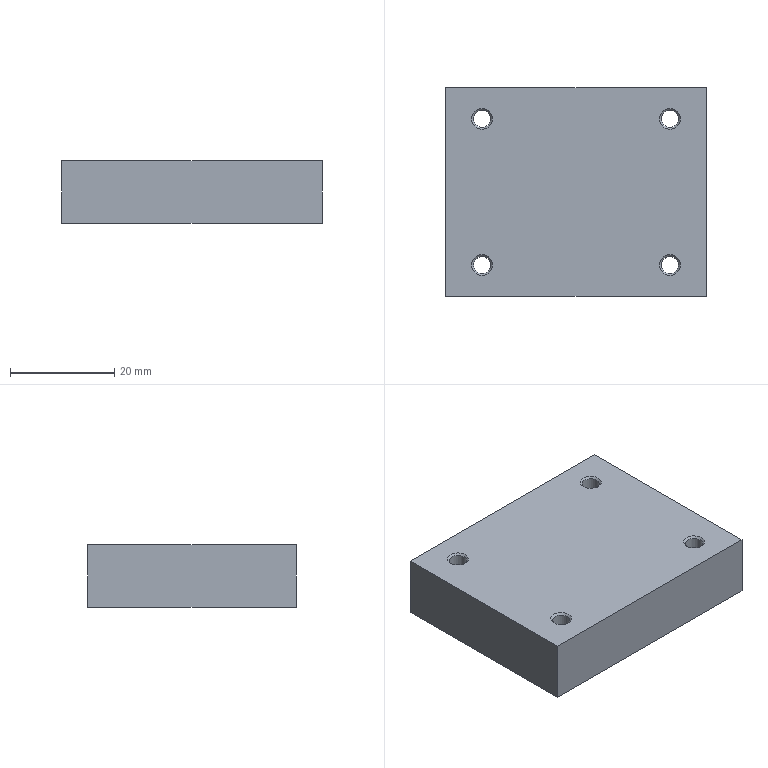Part | NX | features SIMPLE HOLE 4, SYMBOLIC_THREAD 4, DATUM_CSYS 2, BLOCK 1, HOLE PACKAGE 1, SKETCH 1 | 1 solid | 18 faces | box 50 x 40 x 12 mm | volume 23584 mm3 | cone 8 | plane 6 | cylinder 4 | commonest cylinder face diameters 3.3 x4
STEP:
#1=CARTESIAN_POINT('',(45.,34.,12.));
#2=VERTEX_POINT('',#1);
#3=CARTESIAN_POINT('',(43.,34.,12.));
#4=DIRECTION('',(0.,0.,1.));
#5=DIRECTION('',(1.,0.,0.));
#6=AXIS2_PLACEMENT_3D('',#3,#4,#5);
#7=CIRCLE('',#6,2.);
#8=EDGE_CURVE('',#2,#2,#7,.F.);
#9=ORIENTED_EDGE('',*,*,#8,.T.);
#10=EDGE_LOOP('',(#9));
#11=FACE_BOUND('',#10,.T.);
#12=CARTESIAN_POINT('',(45.,6.,12.));
#13=VERTEX_POINT('',#12);
#14=CARTESIAN_POINT('',(43.,6.,12.));
#15=DIRECTION('',(0.,0.,1.));
#16=DIRECTION('',(1.,0.,0.));
#17=AXIS2_PLACEMENT_3D('',#14,#15,#16);
#18=CIRCLE('',#17,2.);
#19=EDGE_CURVE('',#13,#13,#18,.F.);
#20=ORIENTED_EDGE('',*,*,#19,.T.);
#21=EDGE_LOOP('',(#20));
#22=FACE_BOUND('',#21,.T.);
#23=CARTESIAN_POINT('',(9.,34.,12.));
#24=VERTEX_POINT('',#23);
#25=CARTESIAN_POINT('',(7.,34.,12.));
#26=DIRECTION('',(0.,0.,1.));
#27=DIRECTION('',(1.,0.,0.));
#28=AXIS2_PLACEMENT_3D('',#25,#26,#27);
#29=CIRCLE('',#28,2.);
#30=EDGE_CURVE('',#24,#24,#29,.F.);
#31=ORIENTED_EDGE('',*,*,#30,.T.);
#32=EDGE_LOOP('',(#31));
#33=FACE_BOUND('',#32,.T.);
#34=CARTESIAN_POINT('',(9.,6.,12.));
#35=VERTEX_POINT('',#34);
#36=CARTESIAN_POINT('',(7.,6.,12.));
#37=DIRECTION('',(0.,0.,1.));
#38=DIRECTION('',(1.,0.,0.));
#39=AXIS2_PLACEMENT_3D('',#36,#37,#38);
#40=CIRCLE('',#39,2.);
#41=EDGE_CURVE('',#35,#35,#40,.F.);
#42=ORIENTED_EDGE('',*,*,#41,.T.);
#43=EDGE_LOOP('',(#42));
#44=FACE_BOUND('',#43,.T.);
#45=CARTESIAN_POINT('',(50.,0.,12.));
#46=VERTEX_POINT('',#45);
#47=CARTESIAN_POINT('',(0.,0.,12.));
#48=VERTEX_POINT('',#47);
#49=CARTESIAN_POINT('',(25.,0.,12.));
#50=DIRECTION('',(-1.,0.,0.));
#51=VECTOR('',#50,1000.);
#52=LINE('',#49,#51);
#53=EDGE_CURVE('',#46,#48,#52,.T.);
#54=ORIENTED_EDGE('',*,*,#53,.F.);
#55=CARTESIAN_POINT('',(50.,40.,12.));
#56=VERTEX_POINT('',#55);
#57=CARTESIAN_POINT('',(50.,20.,12.));
#58=DIRECTION('',(0.,-1.,0.));
#59=VECTOR('',#58,1000.);
#60=LINE('',#57,#59);
#61=EDGE_CURVE('',#56,#46,#60,.T.);
#62=ORIENTED_EDGE('',*,*,#61,.F.);
#63=CARTESIAN_POINT('',(0.,40.,12.));
#64=VERTEX_POINT('',#63);
#65=CARTESIAN_POINT('',(25.,40.,12.));
#66=DIRECTION('',(1.,0.,0.));
#67=VECTOR('',#66,1000.);
#68=LINE('',#65,#67);
#69=EDGE_CURVE('',#64,#56,#68,.T.);
#70=ORIENTED_EDGE('',*,*,#69,.F.);
#71=CARTESIAN_POINT('',(0.,20.,12.));
#72=DIRECTION('',(0.,1.,0.));
#73=VECTOR('',#72,1000.);
#74=LINE('',#71,#73);
#75=EDGE_CURVE('',#48,#64,#74,.T.);
#76=ORIENTED_EDGE('',*,*,#75,.F.);
#77=EDGE_LOOP('',(#54,#62,#70,#76));
#78=FACE_BOUND('',#77,.T.);
#79=CARTESIAN_POINT('',(25.,20.,12.));
#80=DIRECTION('',(0.,0.,1.));
#81=DIRECTION('',(1.,0.,0.));
#82=AXIS2_PLACEMENT_3D('',#79,#80,#81);
#83=PLANE('',#82);
#84=ADVANCED_FACE('',(#11,#22,#33,#44,#78),#83,.T.);
#85=CARTESIAN_POINT('',(50.,0.,0.));
#86=VERTEX_POINT('',#85);
#87=CARTESIAN_POINT('',(50.,0.,0.));
#88=DIRECTION('',(0.,0.,1.));
#89=VECTOR('',#88,1000.);
#90=LINE('',#87,#89);
#91=EDGE_CURVE('',#86,#46,#90,.T.);
#92=ORIENTED_EDGE('',*,*,#91,.T.);
#93=ORIENTED_EDGE('',*,*,#53,.T.);
#94=CARTESIAN_POINT('',(0.,0.,0.));
#95=VERTEX_POINT('',#94);
#96=CARTESIAN_POINT('',(0.,0.,0.));
#97=DIRECTION('',(0.,0.,1.));
#98=VECTOR('',#97,1000.);
#99=LINE('',#96,#98);
#100=EDGE_CURVE('',#95,#48,#99,.T.);
#101=ORIENTED_EDGE('',*,*,#100,.F.);
#102=CARTESIAN_POINT('',(25.,0.,0.));
#103=DIRECTION('',(1.,0.,0.));
#104=VECTOR('',#103,1000.);
#105=LINE('',#102,#104);
#106=EDGE_CURVE('',#95,#86,#105,.T.);
#107=ORIENTED_EDGE('',*,*,#106,.T.);
#108=EDGE_LOOP('',(#92,#93,#101,#107));
#109=FACE_BOUND('',#108,.T.);
#110=CARTESIAN_POINT('',(25.,0.,0.));
#111=DIRECTION('',(0.,-1.,0.));
#112=DIRECTION('',(0.,0.,-1.));
#113=AXIS2_PLACEMENT_3D('',#110,#111,#112);
#114=PLANE('',#113);
#115=ADVANCED_FACE('',(#109),#114,.T.);
#116=ORIENTED_EDGE('',*,*,#100,.T.);
#117=ORIENTED_EDGE('',*,*,#75,.T.);
#118=CARTESIAN_POINT('',(0.,40.,0.));
#119=VERTEX_POINT('',#118);
#120=CARTESIAN_POINT('',(0.,40.,0.));
#121=DIRECTION('',(0.,0.,1.));
#122=VECTOR('',#121,1000.);
#123=LINE('',#120,#122);
#124=EDGE_CURVE('',#119,#64,#123,.T.);
#125=ORIENTED_EDGE('',*,*,#124,.F.);
#126=CARTESIAN_POINT('',(0.,20.,0.));
#127=DIRECTION('',(0.,-1.,0.));
#128=VECTOR('',#127,1000.);
#129=LINE('',#126,#128);
#130=EDGE_CURVE('',#119,#95,#129,.T.);
#131=ORIENTED_EDGE('',*,*,#130,.T.);
#132=EDGE_LOOP('',(#116,#117,#125,#131));
#133=FACE_BOUND('',#132,.T.);
#134=CARTESIAN_POINT('',(0.,20.,0.));
#135=DIRECTION('',(-1.,0.,0.));
#136=DIRECTION('',(0.,0.,1.));
#137=AXIS2_PLACEMENT_3D('',#134,#135,#136);
#138=PLANE('',#137);
#139=ADVANCED_FACE('',(#133),#138,.T.);
#140=ORIENTED_EDGE('',*,*,#124,.T.);
#141=ORIENTED_EDGE('',*,*,#69,.T.);
#142=CARTESIAN_POINT('',(50.,40.,0.));
#143=VERTEX_POINT('',#142);
#144=CARTESIAN_POINT('',(50.,40.,0.));
#145=DIRECTION('',(0.,0.,1.));
#146=VECTOR('',#145,1000.);
#147=LINE('',#144,#146);
#148=EDGE_CURVE('',#143,#56,#147,.T.);
#149=ORIENTED_EDGE('',*,*,#148,.F.);
#150=CARTESIAN_POINT('',(25.,40.,0.));
#151=DIRECTION('',(-1.,0.,0.));
#152=VECTOR('',#151,1000.);
#153=LINE('',#150,#152);
#154=EDGE_CURVE('',#143,#119,#153,.T.);
#155=ORIENTED_EDGE('',*,*,#154,.T.);
#156=EDGE_LOOP('',(#140,#141,#149,#155));
#157=FACE_BOUND('',#156,.T.);
#158=CARTESIAN_POINT('',(25.,40.,0.));
#159=DIRECTION('',(0.,1.,0.));
#160=DIRECTION('',(0.,0.,1.));
#161=AXIS2_PLACEMENT_3D('',#158,#159,#160);
#162=PLANE('',#161);
#163=ADVANCED_FACE('',(#157),#162,.T.);
#164=CARTESIAN_POINT('',(41.,34.,0.));
#165=VERTEX_POINT('',#164);
#166=CARTESIAN_POINT('',(43.,34.,0.));
#167=DIRECTION('',(0.,0.,-1.));
#168=DIRECTION('',(-1.,0.,0.));
#169=AXIS2_PLACEMENT_3D('',#166,#167,#168);
#170=CIRCLE('',#169,2.);
#171=EDGE_CURVE('',#165,#165,#170,.F.);
#172=ORIENTED_EDGE('',*,*,#171,.T.);
#173=EDGE_LOOP('',(#172));
#174=FACE_BOUND('',#173,.T.);
#175=CARTESIAN_POINT('',(41.,6.,0.));
#176=VERTEX_POINT('',#175);
#177=CARTESIAN_POINT('',(43.,6.,0.));
#178=DIRECTION('',(0.,0.,-1.));
#179=DIRECTION('',(-1.,0.,0.));
#180=AXIS2_PLACEMENT_3D('',#177,#178,#179);
#181=CIRCLE('',#180,2.);
#182=EDGE_CURVE('',#176,#176,#181,.F.);
#183=ORIENTED_EDGE('',*,*,#182,.T.);
#184=EDGE_LOOP('',(#183));
#185=FACE_BOUND('',#184,.T.);
#186=CARTESIAN_POINT('',(5.,34.,0.));
#187=VERTEX_POINT('',#186);
#188=CARTESIAN_POINT('',(7.,34.,0.));
#189=DIRECTION('',(0.,0.,-1.));
#190=DIRECTION('',(-1.,0.,0.));
#191=AXIS2_PLACEMENT_3D('',#188,#189,#190);
#192=CIRCLE('',#191,2.);
#193=EDGE_CURVE('',#187,#187,#192,.F.);
#194=ORIENTED_EDGE('',*,*,#193,.T.);
#195=EDGE_LOOP('',(#194));
#196=FACE_BOUND('',#195,.T.);
#197=CARTESIAN_POINT('',(5.,6.,0.));
#198=VERTEX_POINT('',#197);
#199=CARTESIAN_POINT('',(7.,6.,0.));
#200=DIRECTION('',(0.,0.,-1.));
#201=DIRECTION('',(-1.,0.,0.));
#202=AXIS2_PLACEMENT_3D('',#199,#200,#201);
#203=CIRCLE('',#202,2.);
#204=EDGE_CURVE('',#198,#198,#203,.F.);
#205=ORIENTED_EDGE('',*,*,#204,.T.);
#206=EDGE_LOOP('',(#205));
#207=FACE_BOUND('',#206,.T.);
#208=CARTESIAN_POINT('',(50.,20.,0.));
#209=DIRECTION('',(0.,1.,0.));
#210=VECTOR('',#209,1000.);
#211=LINE('',#208,#210);
#212=EDGE_CURVE('',#86,#143,#211,.T.);
#213=ORIENTED_EDGE('',*,*,#212,.F.);
#214=ORIENTED_EDGE('',*,*,#106,.F.);
#215=ORIENTED_EDGE('',*,*,#130,.F.);
#216=ORIENTED_EDGE('',*,*,#154,.F.);
#217=EDGE_LOOP('',(#213,#214,#215,#216));
#218=FACE_BOUND('',#217,.T.);
#219=CARTESIAN_POINT('',(25.,20.,0.));
#220=DIRECTION('',(0.,0.,-1.));
#221=DIRECTION('',(-1.,0.,0.));
#222=AXIS2_PLACEMENT_3D('',#219,#220,#221);
#223=PLANE('',#222);
#224=ADVANCED_FACE('',(#174,#185,#196,#207,#218),#223,.T.);
#225=ORIENTED_EDGE('',*,*,#212,.T.);
#226=ORIENTED_EDGE('',*,*,#148,.T.);
#227=ORIENTED_EDGE('',*,*,#61,.T.);
#228=ORIENTED_EDGE('',*,*,#91,.F.);
#229=EDGE_LOOP('',(#225,#226,#227,#228));
#230=FACE_BOUND('',#229,.T.);
#231=CARTESIAN_POINT('',(50.,20.,0.));
#232=DIRECTION('',(1.,0.,0.));
#233=DIRECTION('',(0.,0.,-1.));
#234=AXIS2_PLACEMENT_3D('',#231,#232,#233);
#235=PLANE('',#234);
#236=ADVANCED_FACE('',(#230),#235,.T.);
#237=CARTESIAN_POINT('',(5.35,6.,0.35));
#238=VERTEX_POINT('',#237);
#239=CARTESIAN_POINT('',(7.,6.,0.35));
#240=DIRECTION('',(0.,0.,-1.));
#241=DIRECTION('',(-1.,0.,0.));
#242=AXIS2_PLACEMENT_3D('',#239,#240,#241);
#243=CIRCLE('',#242,1.65);
#244=EDGE_CURVE('',#238,#238,#243,.T.);
#245=ORIENTED_EDGE('',*,*,#244,.T.);
#246=EDGE_LOOP('',(#245));
#247=FACE_BOUND('',#246,.T.);
#248=CARTESIAN_POINT('',(8.65,6.,11.65));
#249=VERTEX_POINT('',#248);
#250=CARTESIAN_POINT('',(7.,6.,11.65));
#251=DIRECTION('',(0.,0.,1.));
#252=DIRECTION('',(1.,0.,0.));
#253=AXIS2_PLACEMENT_3D('',#250,#251,#252);
#254=CIRCLE('',#253,1.65);
#255=EDGE_CURVE('',#249,#249,#254,.T.);
#256=ORIENTED_EDGE('',*,*,#255,.T.);
#257=EDGE_LOOP('',(#256));
#258=FACE_BOUND('',#257,.T.);
#259=CARTESIAN_POINT('',(7.,6.,12.));
#260=DIRECTION('',(0.,0.,-1.));
#261=DIRECTION('',(-1.,0.,0.));
#262=AXIS2_PLACEMENT_3D('',#259,#260,#261);
#263=CYLINDRICAL_SURFACE('',#262,1.65);
#264=ADVANCED_FACE('',(#247,#258),#263,.F.);
#265=ORIENTED_EDGE('',*,*,#255,.F.);
#266=EDGE_LOOP('',(#265));
#267=FACE_BOUND('',#266,.T.);
#268=ORIENTED_EDGE('',*,*,#41,.F.);
#269=EDGE_LOOP('',(#268));
#270=FACE_BOUND('',#269,.T.);
#271=CARTESIAN_POINT('',(7.,6.,12.));
#272=DIRECTION('',(0.,0.,1.));
#273=DIRECTION('',(1.,0.,0.));
#274=AXIS2_PLACEMENT_3D('',#271,#272,#273);
#275=CONICAL_SURFACE('',#274,2.,0.7854);
#276=ADVANCED_FACE('',(#267,#270),#275,.F.);
#277=ORIENTED_EDGE('',*,*,#204,.F.);
#278=EDGE_LOOP('',(#277));
#279=FACE_BOUND('',#278,.T.);
#280=ORIENTED_EDGE('',*,*,#244,.F.);
#281=EDGE_LOOP('',(#280));
#282=FACE_BOUND('',#281,.T.);
#283=CARTESIAN_POINT('',(7.,6.,0.35));
#284=DIRECTION('',(0.,0.,-1.));
#285=DIRECTION('',(-1.,0.,0.));
#286=AXIS2_PLACEMENT_3D('',#283,#284,#285);
#287=CONICAL_SURFACE('',#286,1.65,0.7854);
#288=ADVANCED_FACE('',(#279,#282),#287,.F.);
#289=CARTESIAN_POINT('',(5.35,34.,0.35));
#290=VERTEX_POINT('',#289);
#291=CARTESIAN_POINT('',(7.,34.,0.35));
#292=DIRECTION('',(0.,0.,-1.));
#293=DIRECTION('',(-1.,0.,0.));
#294=AXIS2_PLACEMENT_3D('',#291,#292,#293);
#295=CIRCLE('',#294,1.65);
#296=EDGE_CURVE('',#290,#290,#295,.T.);
#297=ORIENTED_EDGE('',*,*,#296,.T.);
#298=EDGE_LOOP('',(#297));
#299=FACE_BOUND('',#298,.T.);
#300=CARTESIAN_POINT('',(8.65,34.,11.65));
#301=VERTEX_POINT('',#300);
#302=CARTESIAN_POINT('',(7.,34.,11.65));
#303=DIRECTION('',(0.,0.,1.));
#304=DIRECTION('',(1.,0.,0.));
#305=AXIS2_PLACEMENT_3D('',#302,#303,#304);
#306=CIRCLE('',#305,1.65);
#307=EDGE_CURVE('',#301,#301,#306,.T.);
#308=ORIENTED_EDGE('',*,*,#307,.T.);
#309=EDGE_LOOP('',(#308));
#310=FACE_BOUND('',#309,.T.);
#311=CARTESIAN_POINT('',(7.,34.,12.));
#312=DIRECTION('',(0.,0.,-1.));
#313=DIRECTION('',(-1.,0.,0.));
#314=AXIS2_PLACEMENT_3D('',#311,#312,#313);
#315=CYLINDRICAL_SURFACE('',#314,1.65);
#316=ADVANCED_FACE('',(#299,#310),#315,.F.);
#317=ORIENTED_EDGE('',*,*,#307,.F.);
#318=EDGE_LOOP('',(#317));
#319=FACE_BOUND('',#318,.T.);
#320=ORIENTED_EDGE('',*,*,#30,.F.);
#321=EDGE_LOOP('',(#320));
#322=FACE_BOUND('',#321,.T.);
#323=CARTESIAN_POINT('',(7.,34.,12.));
#324=DIRECTION('',(0.,0.,1.));
#325=DIRECTION('',(1.,0.,0.));
#326=AXIS2_PLACEMENT_3D('',#323,#324,#325);
#327=CONICAL_SURFACE('',#326,2.,0.7854);
#328=ADVANCED_FACE('',(#319,#322),#327,.F.);
#329=ORIENTED_EDGE('',*,*,#193,.F.);
#330=EDGE_LOOP('',(#329));
#331=FACE_BOUND('',#330,.T.);
#332=ORIENTED_EDGE('',*,*,#296,.F.);
#333=EDGE_LOOP('',(#332));
#334=FACE_BOUND('',#333,.T.);
#335=CARTESIAN_POINT('',(7.,34.,0.35));
#336=DIRECTION('',(0.,0.,-1.));
#337=DIRECTION('',(-1.,0.,0.));
#338=AXIS2_PLACEMENT_3D('',#335,#336,#337);
#339=CONICAL_SURFACE('',#338,1.65,0.7854);
#340=ADVANCED_FACE('',(#331,#334),#339,.F.);
#341=CARTESIAN_POINT('',(41.35,6.,0.35));
#342=VERTEX_POINT('',#341);
#343=CARTESIAN_POINT('',(43.,6.,0.35));
#344=DIRECTION('',(0.,0.,-1.));
#345=DIRECTION('',(-1.,0.,0.));
#346=AXIS2_PLACEMENT_3D('',#343,#344,#345);
#347=CIRCLE('',#346,1.65);
#348=EDGE_CURVE('',#342,#342,#347,.T.);
#349=ORIENTED_EDGE('',*,*,#348,.T.);
#350=EDGE_LOOP('',(#349));
#351=FACE_BOUND('',#350,.T.);
#352=CARTESIAN_POINT('',(44.65,6.,11.65));
#353=VERTEX_POINT('',#352);
#354=CARTESIAN_POINT('',(43.,6.,11.65));
#355=DIRECTION('',(0.,0.,1.));
#356=DIRECTION('',(1.,0.,0.));
#357=AXIS2_PLACEMENT_3D('',#354,#355,#356);
#358=CIRCLE('',#357,1.65);
#359=EDGE_CURVE('',#353,#353,#358,.T.);
#360=ORIENTED_EDGE('',*,*,#359,.T.);
#361=EDGE_LOOP('',(#360));
#362=FACE_BOUND('',#361,.T.);
#363=CARTESIAN_POINT('',(43.,6.,12.));
#364=DIRECTION('',(0.,0.,-1.));
#365=DIRECTION('',(-1.,0.,0.));
#366=AXIS2_PLACEMENT_3D('',#363,#364,#365);
#367=CYLINDRICAL_SURFACE('',#366,1.65);
#368=ADVANCED_FACE('',(#351,#362),#367,.F.);
#369=ORIENTED_EDGE('',*,*,#359,.F.);
#370=EDGE_LOOP('',(#369));
#371=FACE_BOUND('',#370,.T.);
#372=ORIENTED_EDGE('',*,*,#19,.F.);
#373=EDGE_LOOP('',(#372));
#374=FACE_BOUND('',#373,.T.);
#375=CARTESIAN_POINT('',(43.,6.,12.));
#376=DIRECTION('',(0.,0.,1.));
#377=DIRECTION('',(1.,0.,0.));
#378=AXIS2_PLACEMENT_3D('',#375,#376,#377);
#379=CONICAL_SURFACE('',#378,2.,0.7854);
#380=ADVANCED_FACE('',(#371,#374),#379,.F.);
#381=ORIENTED_EDGE('',*,*,#182,.F.);
#382=EDGE_LOOP('',(#381));
#383=FACE_BOUND('',#382,.T.);
#384=ORIENTED_EDGE('',*,*,#348,.F.);
#385=EDGE_LOOP('',(#384));
#386=FACE_BOUND('',#385,.T.);
#387=CARTESIAN_POINT('',(43.,6.,0.35));
#388=DIRECTION('',(0.,0.,-1.));
#389=DIRECTION('',(-1.,0.,0.));
#390=AXIS2_PLACEMENT_3D('',#387,#388,#389);
#391=CONICAL_SURFACE('',#390,1.65,0.7854);
#392=ADVANCED_FACE('',(#383,#386),#391,.F.);
#393=CARTESIAN_POINT('',(41.35,34.,0.35));
#394=VERTEX_POINT('',#393);
#395=CARTESIAN_POINT('',(43.,34.,0.35));
#396=DIRECTION('',(0.,0.,-1.));
#397=DIRECTION('',(-1.,0.,0.));
#398=AXIS2_PLACEMENT_3D('',#395,#396,#397);
#399=CIRCLE('',#398,1.65);
#400=EDGE_CURVE('',#394,#394,#399,.T.);
#401=ORIENTED_EDGE('',*,*,#400,.T.);
#402=EDGE_LOOP('',(#401));
#403=FACE_BOUND('',#402,.T.);
#404=CARTESIAN_POINT('',(44.65,34.,11.65));
#405=VERTEX_POINT('',#404);
#406=CARTESIAN_POINT('',(43.,34.,11.65));
#407=DIRECTION('',(0.,0.,1.));
#408=DIRECTION('',(1.,0.,0.));
#409=AXIS2_PLACEMENT_3D('',#406,#407,#408);
#410=CIRCLE('',#409,1.65);
#411=EDGE_CURVE('',#405,#405,#410,.T.);
#412=ORIENTED_EDGE('',*,*,#411,.T.);
#413=EDGE_LOOP('',(#412));
#414=FACE_BOUND('',#413,.T.);
#415=CARTESIAN_POINT('',(43.,34.,12.));
#416=DIRECTION('',(0.,0.,-1.));
#417=DIRECTION('',(-1.,0.,0.));
#418=AXIS2_PLACEMENT_3D('',#415,#416,#417);
#419=CYLINDRICAL_SURFACE('',#418,1.65);
#420=ADVANCED_FACE('',(#403,#414),#419,.F.);
#421=ORIENTED_EDGE('',*,*,#411,.F.);
#422=EDGE_LOOP('',(#421));
#423=FACE_BOUND('',#422,.T.);
#424=ORIENTED_EDGE('',*,*,#8,.F.);
#425=EDGE_LOOP('',(#424));
#426=FACE_BOUND('',#425,.T.);
#427=CARTESIAN_POINT('',(43.,34.,12.));
#428=DIRECTION('',(0.,0.,1.));
#429=DIRECTION('',(1.,0.,0.));
#430=AXIS2_PLACEMENT_3D('',#427,#428,#429);
#431=CONICAL_SURFACE('',#430,2.,0.7854);
#432=ADVANCED_FACE('',(#423,#426),#431,.F.);
#433=ORIENTED_EDGE('',*,*,#171,.F.);
#434=EDGE_LOOP('',(#433));
#435=FACE_BOUND('',#434,.T.);
#436=ORIENTED_EDGE('',*,*,#400,.F.);
#437=EDGE_LOOP('',(#436));
#438=FACE_BOUND('',#437,.T.);
#439=CARTESIAN_POINT('',(43.,34.,0.35));
#440=DIRECTION('',(0.,0.,-1.));
#441=DIRECTION('',(-1.,0.,0.));
#442=AXIS2_PLACEMENT_3D('',#439,#440,#441);
#443=CONICAL_SURFACE('',#442,1.65,0.7854);
#444=ADVANCED_FACE('',(#435,#438),#443,.F.);
#445=CLOSED_SHELL('',(#84,#115,#139,#163,#224,#236,#264,#276,#288,#316,#328,#340,#368,#380,#392,#420,#432,#444));
#446=MANIFOLD_SOLID_BREP('',#445);
#447=(LENGTH_UNIT()NAMED_UNIT(*)SI_UNIT(.MILLI.,.METRE.));
#448=UNCERTAINTY_MEASURE_WITH_UNIT(LENGTH_MEASURE(0.00001),#447,'','');
#449=(NAMED_UNIT(*)PLANE_ANGLE_UNIT()SI_UNIT($,.RADIAN.));
#450=(NAMED_UNIT(*)SI_UNIT($,.STERADIAN.)SOLID_ANGLE_UNIT());
#451=(GEOMETRIC_REPRESENTATION_CONTEXT(3)GLOBAL_UNCERTAINTY_ASSIGNED_CONTEXT((#448))GLOBAL_UNIT_ASSIGNED_CONTEXT((#447,#449,#450))REPRESENTATION_CONTEXT('',''));
#452=ADVANCED_BREP_SHAPE_REPRESENTATION('',(#446),#451);